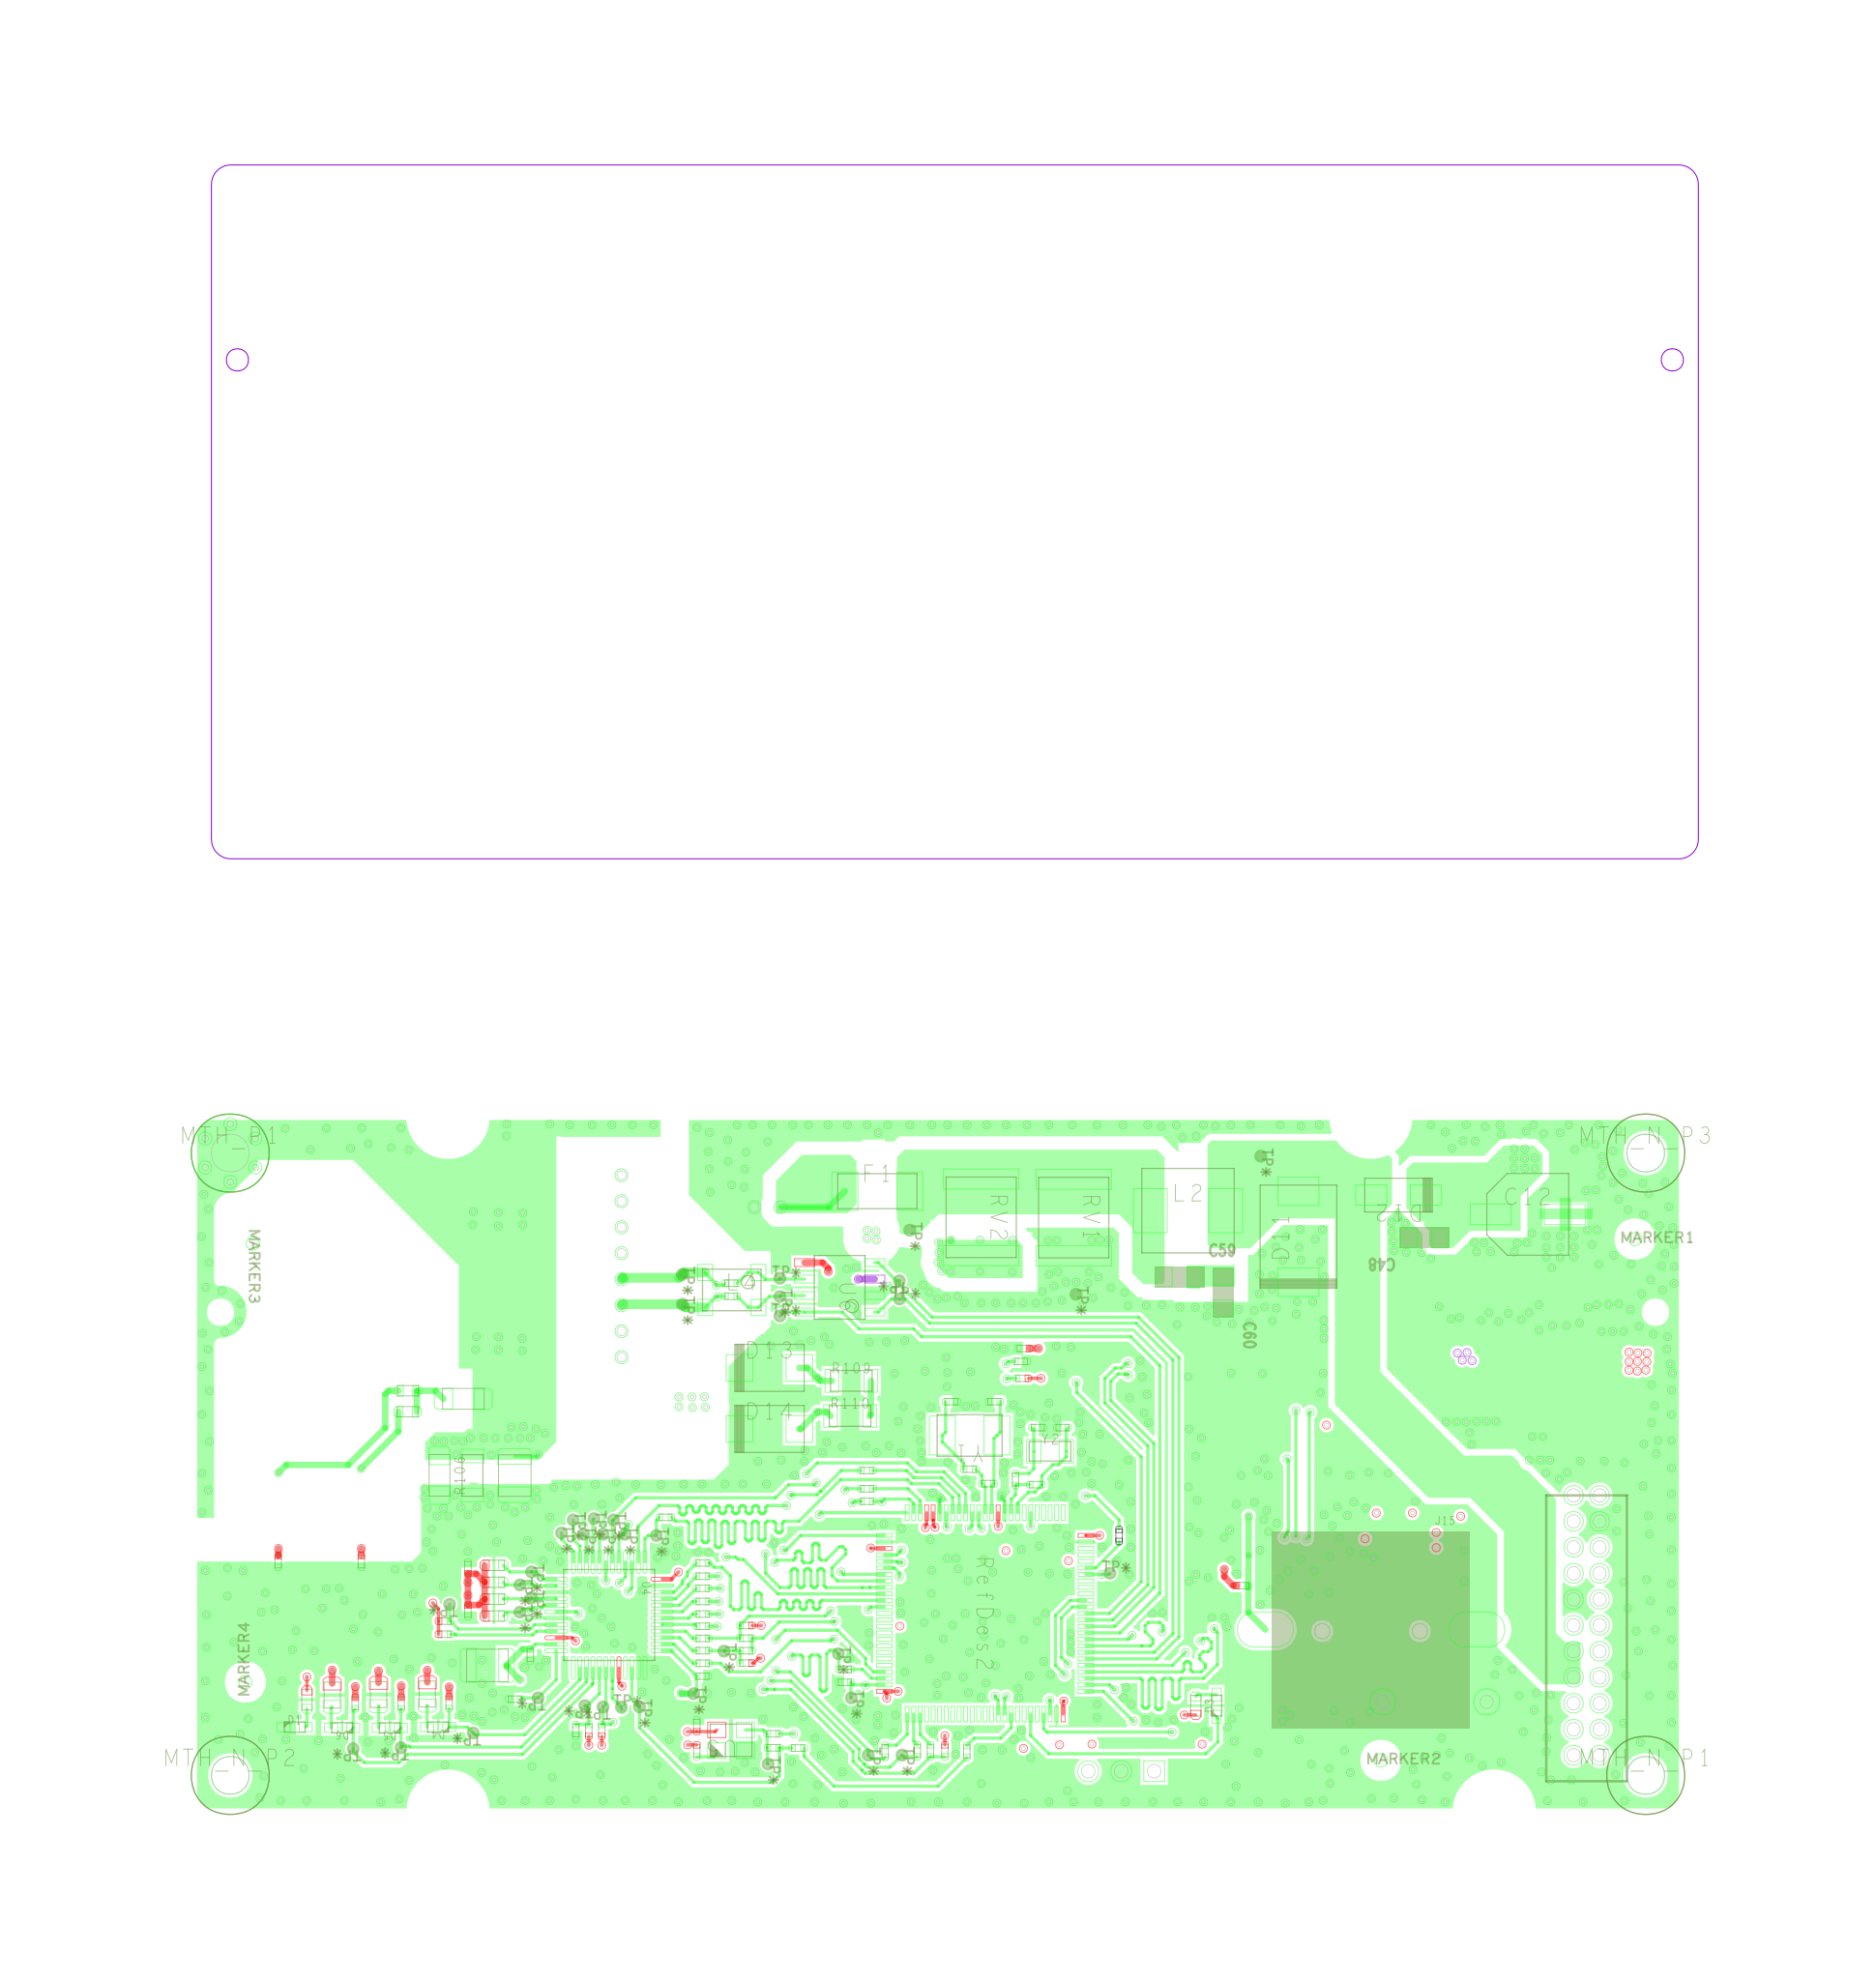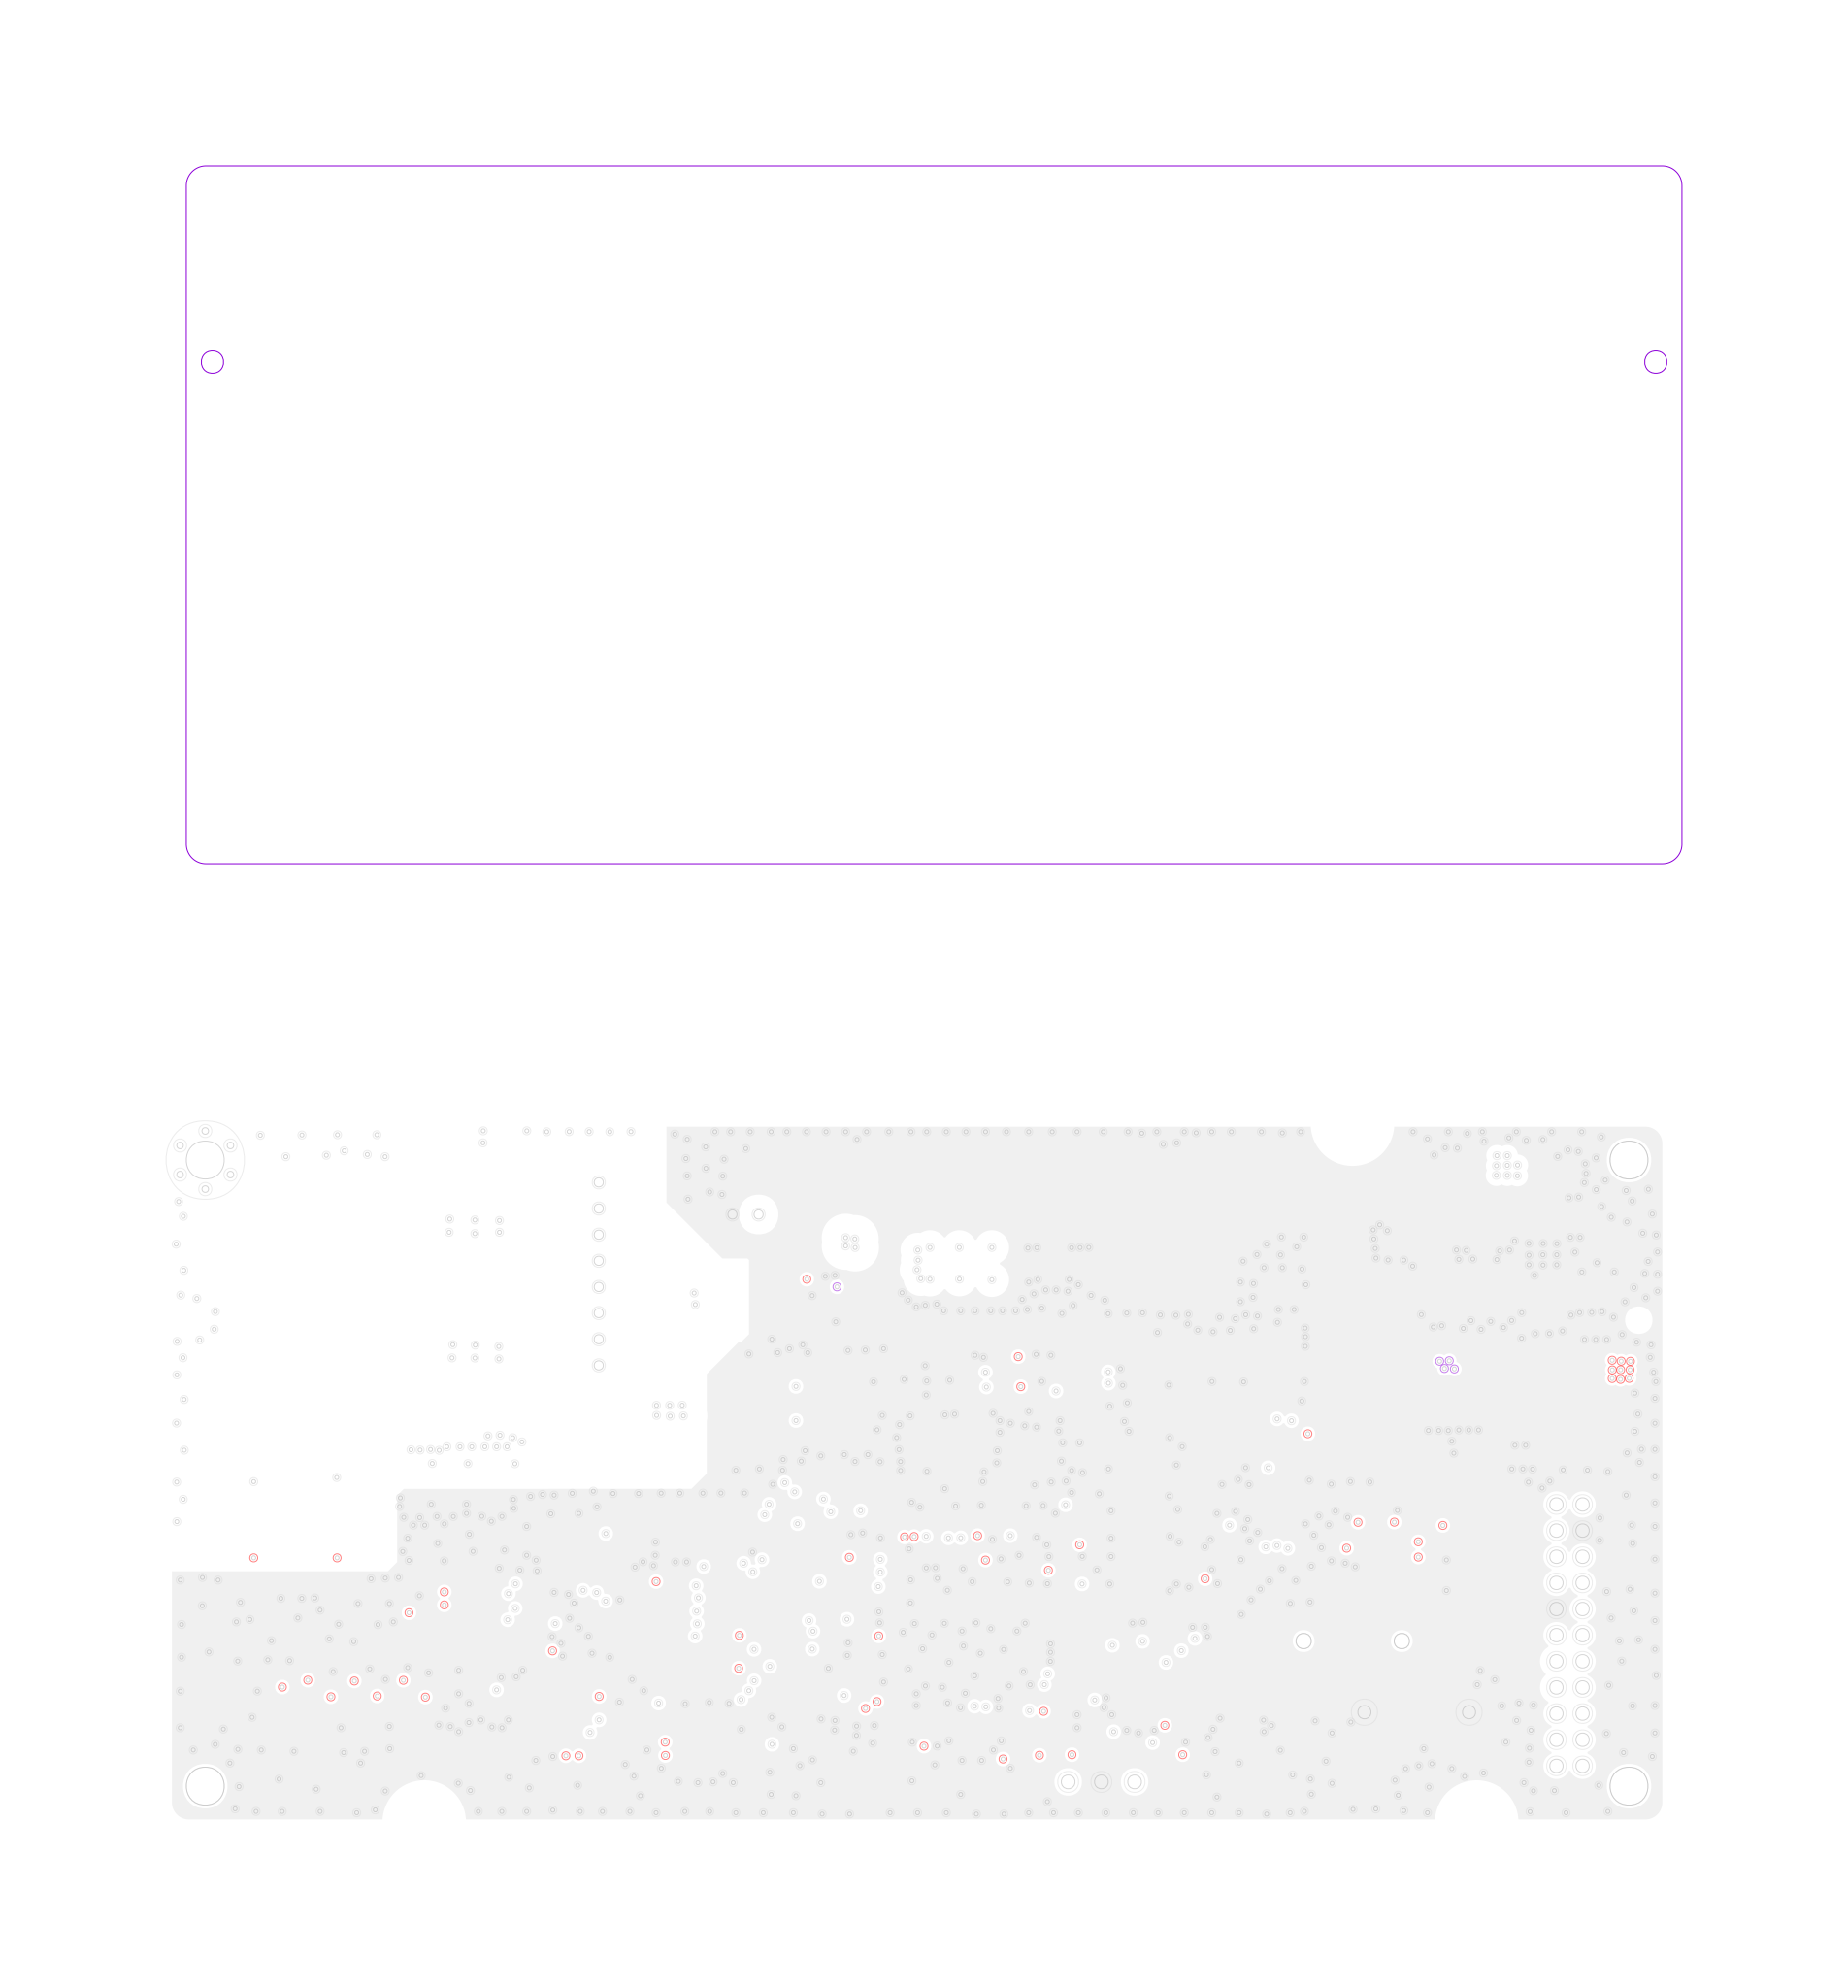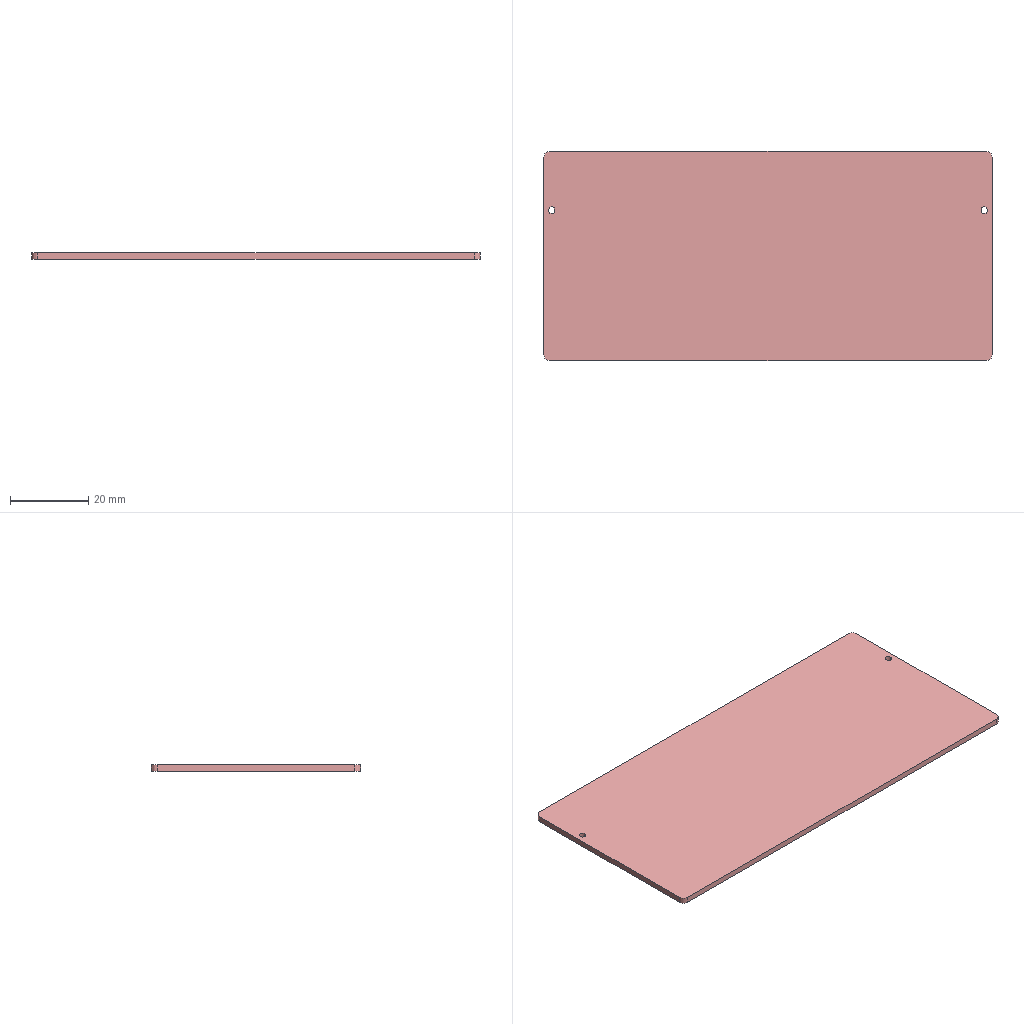Circuit board layout | Cadence Allegro | box 114.4 x 53.4 x 1.5 mm
Layer stack:
# Cadence Allegro layer stack of  (unit mm; from the constraint file cross-section; dielectric type: 0 not recorded (Allegro does not mark core vs prepreg), 3 surface material)
index,name,kind,layer,copper_thickness_mm,dielectric_type,dielectric_thickness_mm,dielectric_material,dielectric_constant
0,Top Surface,other,,,,,,
1,TOP,copper,TOP,0.03,,,,
2,Dielectric1,dielectric,,,0,0.5,FR-4,4.5
3,GND,copper,GND,0.03,,,,
4,Dielectric2,dielectric,,,0,0.5,FR-4,4.5
5,POWER,copper,POWER,0.03,,,,
6,Dielectric3,dielectric,,,0,0.48,FR-4,4.5
7,BOTTOM,copper,BOTTOM,0.03,,,,
8,Bottom Surface,other,,,,,,
# drill layer pairs: low layer,high layer
drill_pair,TOP,BOTTOM
Part placement:
REFDES,COMP_VALUE,SYM_NAME,SYM_X,SYM_Y,SYM_ROTATE,SYM_MIRROR
C1,8PF,C0402,154.5,96.5,180.000,NO
C2,8PF,C0402,157.8,96.5,0.000,NO
C3,6PF,C0402,161.145,94.5,0.000,NO
C4,6PF,C0402,163.045,94.5,180.000,NO
C6,22uf,C1210,192.63,95.39,90.000,YES
C7,22uf,C1210,187.28,101.31,0.000,YES
C8,.22uf,C0805,195.197,115.26,0.000,YES
C9,.1uf,C0402,193.15,101.71,270.000,YES
C10,4.7uf,C1210,202.062,114.475,180.000,YES
C11,.1uf,C0402,195.347,112.262,0.000,YES
C12,47uF,CAPAE630X770N,198.84,110.92,0.000,NO
C13,.1uf,C0402,160.058,100.595,180.000,NO
C14,10uf,C1210,118.8,76.2,180.000,NO
C15,.1uf,C0402,122.1,77,270.000,NO
C16,.1uf,C0402,145.6,107.2,180.000,YES
C17,.1uf,C0402,134.907,71.552,90.000,NO
C18,.1uf,C0402,125.6,71.2,270.000,NO
C19,10uf,C1210,196.08,95.43,90.000,YES
C20,1uf,C0603,194.39,101.9,270.000,YES
C21,.1uf,C0402,156.977,85.515,90.000,YES
C22,.1uf,C0402,191.8,87.47,270.000,YES
C23,2.2uf,C0603,185.52,87,0.000,YES
C24,.1uf,C0402,153.4,88,270.000,YES
C25,1uf,C0603,152.3,88.4,270.000,YES
C26,.1uf,C0402,164.7,86.2,0.000,YES
C27,.1uf,C0402,102.7,84.2,270.000,NO
C28,.1uf,C0402,158.088,88.097,270.000,YES
C29,.1uf,C0402,149.425,85.51,180.000,YES
C30,.1uf,C0402,153.936,85.518,90.000,YES
C31,.047uf,C0402,151.857,85.886,180.000,YES
C32,.047uf,C0402,151.857,81.745,180.000,YES
C33,.1uf,C0402,109.1,84.2,270.000,NO
C34,.047uf,C0402,151.84,83.793,180.000,YES
C35,.1uf,C0402,183.355,93.62,90.000,YES
C36,22uf,C1210,204.92,101.46,270.000,YES
C37,10uf,C1210,131.723,84.653,270.000,YES
C38,2.2uf,C0603,148.002,72.98,90.000,YES
C39,.1uf,C0402,134.301,84.145,270.000,YES
C40,.1uf,C0402,117.3,80.4,270.000,NO
C41,.1uf,C0402,149.518,72.64,90.000,YES
C42,.047uf,C0402,171.928,84.672,270.000,YES
C43,10uf,C1210,153.02,73.522,180.000,YES
C44,.1uf,C0402,162.54,72.507,0.000,YES
C45,.1uf,C0402,125.8,81.3,270.000,YES
C46,.1uf,C0402,117.3,83.7,90.000,NO
C47,2.2uf,C0603,161.285,74.382,0.000,YES
C48,.1uf,C0805,190.9,109.1,180.000,NO
C49,.1uf,C0402,124.484,77.668,0.000,YES
C50,.1uf,C0402,135.347,75.368,0.000,NO
C51,.1uf,C0402,129.637,73.805,180.000,YES
C52,1.5nF,C1206,116.948,96.718,0.000,NO
C53,47nf,C1210,120.903,90.81,90.000,NO
C54,.1uf,C0402,146.24,105.933,180.000,YES
C55,4700pf(NC),C0603,138.657,103.775,90.000,YES
C56,10nF,C1206,115.115,90.828,90.000,NO
C57,100PF,C0603,145.958,102.522,180.000,YES
C58,100PF,C0603,145.972,103.96,180.000,YES
C59,.1uf,C0805,172.048,106.11,0.000,NO
C60,.1uf,C0805,175.405,104.897,270.000,NO
D1,LED,LED0603,103.97,71.448,0.000,NO
D2,UFS08A2.8L04,SOIC127P600X175-8N,105.108,100.885,270.000,YES
D3,LED,LED0603,174.9,73.1,90.000,NO
D4,LED,LED0603,115.01,71.45,180.000,NO
D5,LED,LED0603,111.287,71.387,180.000,NO
D6,LED,LED0603,107.625,71.395,180.000,NO
D8,SMBJ10CA,SMB,147.205,97.103,270.000,YES
D9,SS26FL,SMA,199.49,100.78,180.000,YES
D10,SS26FL,SMA,196.67,107.65,270.000,YES
D11,TPSMC27CA,SMC,181.2,109.2,90.000,NO
D12,NRVA4007T3G,SMA,188.9,112.4,180.000,NO
D13,SMBJ10CA,SMB,140.5,99.1,0.000,NO
D14,SMBJ10CA,SMB,140.5,94.4,0.000,NO
F1,10A,FUSE10A,148.8,112.7,0.000,NO
GDT1,5kA,GDT5KA2P,152.705,108.942,0.000,YES
J15,BAT2,CR1220,186.785,78.834,0.000,NO
J17,532530870,532530870,129.116,106.926,180.000,YES
J18,532530270,532530270,140.342,111.471,270.000,YES
J19,2x11,CON2X11X200,202.366,69.286,90.000,NO
J20,3,CON3X254,170.1,68.06,0.000,YES
L1,6.8uH,SPM5030,191.18,106.38,0.000,YES
L2,22uH,SPM6530,172.7,111.2,0.000,NO
L3,51uH,CM320X450X150-4N,154.243,98.785,270.000,YES
L4,51uH,CM320X450X150-4N,137.6,105.1,270.000,NO
MARKER1,30mil,FIDMS0,207.09,109.02,0.000,NO
MARKER2,30mil,FIDMS0,187.54,68.89,0.000,NO
MARKER3,30mil,FIDMS0,100.75,108.67,270.000,NO
MARKER4,30mil,FIDMS0,100.18,74.918,90.000,NO
MARKER5,30mil,FIDMS0,185.08,112.74,0.000,YES
MARKER6,30mil,FIDMS0,178.09,71.59,270.000,YES
MARKER7,30mil,FIDMS0,100.75,108.65,0.000,YES
MARKER8,30mil,FIDMS0,100.18,74.918,0.000,YES
MTH_N_P1,D2.8no-plated,MTGNP600H280Z380P,207.916,67.736,0.000,NO
MTH_N_P2,D2.8no-plated,MTGNP600H280Z380P,99.016,67.736,0.000,NO
MTH_N_P3,D2.8no-plated,MTGNP600H280Z380P,207.916,115.636,0.000,NO
MTH_P1,D2.8plated,MTGP6000H280V6P,99.016,115.636,0.000,NO
R1,0R(NC),R0402,176.88,82.34,180.000,NO
R2,10k,R0402,190.7,87.47,90.000,YES
R3,10k,R0402,192.9,87.47,90.000,YES
R4,10k,R0402,194.7,87.47,90.000,YES
R5,10k,R0402,196.2,87.47,90.000,YES
R6,10k,R0402,189.3,87.47,90.000,YES
R7,10k,R0402,187.9,87.47,90.000,YES
R8,10k,R0402,200.542,103.71,90.000,YES
R9,68k,R0402,201.59,103.705,270.000,YES
R10,12k,R0402,202.635,103.72,90.000,YES
R11,16.9k,R0402,205.412,111.22,180.000,YES
R12,33R,R0402,148,91.2,180.000,NO
R13,0R,R0402,155.9,91.3,0.000,NO
R14,1k,R0603,104.912,73.565,270.000,NO
R15,1M,R0402,157.31,90.188,180.000,NO
R16,10M,R0402,160.99,90.112,0.000,NO
R17,0R,R0402,148,89.8,180.000,NO
R18,10k,R0402,197.7,87.47,90.000,YES
R19,0R,R0402,148.002,88.828,180.000,NO
R20,33R,R0402,132.5,87.6,180.000,NO
R21,33R,R0402,146.3,75.9,180.000,NO
R22,33R,R0402,135.351,84.081,180.000,NO
R23,0R(NC),R0402,146.3,74.9,180.000,NO
R24,33R,R0402,135.351,83.065,180.000,NO
R25,33R,R0402,135.351,82.138,180.000,NO
R26,2.2k,R0402,138.703,79.269,180.000,NO
R27,33R,R0402,135.351,81.122,180.000,NO
R28,0R,R0402,140.778,70.935,180.000,NO
R29,0R,R0402,138.703,78.294,180.000,NO
R30,33R,R0402,135.357,78.28,180.000,NO
R31,33R,R0402,149.4,69.6,270.000,NO
R32,33R,R0402,151.872,69.626,270.000,NO
R33,0R,R0402,152.888,69.626,90.000,NO
R34,10k,R0402,153.993,69.626,270.000,NO
R35,33R,R0402,155.683,69.575,90.000,NO
R36,0R,R0402,140.8,69.858,0.000,NO
R37,0R,R0402,138.703,77.329,180.000,NO
R38,33R,R0402,135.359,77.336,180.000,NO
R39,2.2k,R0402,138.703,76.376,180.000,NO
R40,33R,R0402,135.364,76.367,180.000,NO
R41,10k,R0402,159.958,98.295,180.000,NO
R42,10k,R0402,159.857,99.595,180.000,NO
R43,2.2k,R0402,115.5,78.6,180.000,NO
R44,2.2k,R0402,115.5,79.6,180.000,NO
R45,10k,R0402,134.907,69.62,90.000,NO
R46,0R,R0402,142.7,69.84,180.000,NO
R47,4.87k,R0402,120.9,73.6,180.000,NO
R48,10k,R0402,126.6,71.2,90.000,NO
R49,1.5k,R0402,127.6,71.2,90.000,NO
R50,4.7R,R1206,112.912,113.02,180.000,YES
R51,4.7R,R1206,112.907,109.525,180.000,YES
R52,4.7R,R1206,112.862,104.265,180.000,YES
R53,4.7R,R1206,112.88,100.933,180.000,YES
R57,10k,R0402,173.1,70.6,270.000,YES
R60,10k,R0402,168.78,70.6,90.000,YES
R62,10k,R0402,166,70.6,270.000,YES
R63,10k,R0402,163.5,70.6,270.000,YES
R65,10k,R0402,161,70.6,270.000,YES
R67,10k,R0402,158.018,85.49,270.000,YES
R68,0R,R0402,154.438,87.99,90.000,YES
R69,0R(NC),R0402,154.952,85.518,90.000,YES
R70,10k,R0402,164.708,84.25,180.000,YES
R71,1k,R0402,151.857,84.82,180.000,YES
R72,10k(NC),R0402,164.7,83.23,0.000,YES
R73,33R,R0402,167.4,86.2,90.000,NO
R74,1k,R0402,151.9,80.7,180.000,YES
R75,1k,R0402,190.67,112.32,90.000,YES
R76,10k,R0402,191.78,112.34,90.000,YES
R77,1k,R0402,185.591,96.978,180.000,YES
R78,10k,R0402,187.489,96.991,0.000,YES
R79,10k,R0402,181.197,93.612,270.000,YES
R80,1k,R0402,151.847,82.772,180.000,YES
R81,10k,R0402,182.23,93.605,90.000,YES
R82,10k(NC),R0402,149.385,79.225,0.000,YES
R83,10k,R0402,149.377,80.228,180.000,YES
R84,49.9R,R0603,119.3,83.9,180.000,NO
R85,49.9R,R0603,119.3,82.6,180.000,NO
R86,49.9R,R0603,119.3,81.3,180.000,NO
R87,1k,R0402,173.04,84.707,270.000,YES
R88,10k,R0402,175.037,84.692,270.000,YES
R89,49.9R,R0603,119.3,80,180.000,NO
R90,33R,R0402,135.36,80.153,180.000,NO
R91,75R,R0603,112.657,95.728,0.000,NO
R92,75R,R0603,112.695,97.34,0.000,NO
R93,1k,R0402,174.042,84.7,270.000,YES
R94,33R,R0402,135.363,79.213,180.000,NO
R95,1k,R0603,173.3,73.1,90.000,NO
R96,2.2k,R0402,115.855,73.335,90.000,NO
R97,390R,R0805,114.17,74,90.000,NO
R98,2.2k,R0402,112.17,73.295,90.000,NO
R99,390R,R0805,110.422,73.957,90.000,NO
R101,62R(NC),R1206,142.12,105.112,0.000,YES
R102,62R(NC),R1206,142.12,102.705,0.000,YES
R103,2.2k,R0402,108.63,73.293,90.000,NO
R104,390R,R0805,106.86,73.907,90.000,NO
R106,1M,R1206,117.655,90.82,90.000,NO
R109,62R,R1206,146.8,98.1,0.000,NO
R110,62R,R1206,146.7,95.4,0.000,NO
R111,4.7R,R1206,141.852,98.315,0.000,YES
R112,4.7R,R1206,141.882,95.705,0.000,YES
R113,10R,R0402,159.43,90.507,90.000,NO
R114,0R(NC),R0402,137.555,105.618,180.000,NO
R115,0R(NC),R0402,137.545,104.61,180.000,NO
RT1,10K,R0603,179.425,93.045,0.000,YES
RV1,47V,R2220,163.905,110.668,270.000,NO
RV2,47V,R2220,156.79,110.69,270.000,NO
RV3,47V,R2220,160.925,108.942,180.000,YES
T1,HR641680E,H1102,105.897,88.26,270.000,YES
TF1,TF-01A,TF-01A,198.49,73.39,0.000,YES
TP1,TP,TPAD_30MIL,164.084,104.763,270.000,NO
TP2,TP,TPAD_30MIL,184.827,94.356,180.000,YES
TP3,TP,TPAD_30MIL,205.374,105.758,180.000,YES
TP4,TP,TPAD_30MIL,205.256,109.746,90.000,YES
TP5,TP,TPAD_30MIL,194.801,85.766,90.000,YES
TP6,TP,TPAD_30MIL,190.699,85.774,270.000,YES
TP7,TP,TPAD_30MIL,187.899,85.874,270.000,YES
TP8,TP,TPAD_30MIL,192.904,85.871,180.000,YES
TP9,TP,TPAD_30MIL,189.299,85.874,270.000,YES
TP10,TP,TPAD_30MIL,196.199,85.774,270.000,YES
TP11,TP,TPAD_30MIL,129.399,86.296,270.000,NO
TP12,TP,TPAD_30MIL,198.161,113.814,180.000,YES
TP13,TP,TPAD_30MIL,156.804,87.669,90.000,YES
TP14,TP,TPAD_30MIL,193.149,98.794,270.000,YES
TP15,TP,TPAD_30MIL,197.699,85.774,270.000,YES
TP16,TP,TPAD_30MIL,102.838,96.323,90.000,YES
TP17,TP,TPAD_30MIL,197.288,112.183,90.000,YES
TP18,TP,TPAD_30MIL,104.328,96.31,90.000,YES
TP19,TP,TPAD_30MIL,193.681,112.196,90.000,YES
TP20,TP,TPAD_30MIL,166.704,83.299,0.000,NO
TP21,TP,TPAD_30MIL,105.828,96.26,90.000,YES
TP22,TP,TPAD_30MIL,167.161,99.296,180.000,YES
TP23,TP,TPAD_30MIL,167.462,100.696,180.000,YES
TP24,TP,TPAD_30MIL,107.255,96.272,90.000,YES
TP25,TP,TPAD_30MIL,126.999,87.496,270.000,NO
TP26,TP,TPAD_30MIL,127.699,86.296,270.000,NO
TP27,TP,TPAD_30MIL,167.357,97.699,270.000,YES
TP28,TP,TPAD_30MIL,126.199,86.296,270.000,NO
TP29,TP,TPAD_30MIL,145.799,77.096,270.000,NO
TP30,TP,TPAD_30MIL,125.399,87.396,270.000,NO
TP31,TP,TPAD_30MIL,128.499,87.396,270.000,NO
TP32,TP,TPAD_30MIL,124.499,86.396,270.000,NO
TP33,TP,TPAD_30MIL,133.799,106.296,270.000,NO
TP34,TP,TPAD_30MIL,131.799,86.196,270.000,NO
TP35,TP,TPAD_30MIL,122.199,83.396,270.000,NO
TP36,TP,TPAD_30MIL,121.299,82.396,270.000,NO
TP37,TP,TPAD_30MIL,122.199,81.396,270.000,NO
TP38,TP,TPAD_30MIL,178.299,115.396,270.000,NO
TP39,TP,TPAD_30MIL,121.299,80.296,270.000,NO
TP40,TP,TPAD_30MIL,133.799,103.996,270.000,NO
TP41,TP,TPAD_30MIL,146.799,73.696,270.000,NO
TP42,TP,TPAD_30MIL,186.001,95.744,270.000,YES
TP43,TP,TPAD_30MIL,182.201,91.919,0.000,YES
TP44,TP,TPAD_30MIL,163.416,74.351,90.000,YES
TP45,TP,TPAD_30MIL,189.276,111.949,0.000,YES
TP46,TP,TPAD_30MIL,176.369,85.199,0.000,YES
TP47,TP,TPAD_30MIL,157.999,98.004,270.000,YES
TP48,TP,TPAD_30MIL,136.999,77.296,270.000,NO
TP49,TP,TPAD_30MIL,130.499,72.996,270.000,NO
TP50,TP,TPAD_30MIL,150.699,69.296,270.000,NO
TP51,TP,TPAD_30MIL,148.099,69.296,270.000,NO
TP52,TP,TPAD_30MIL,150.496,105.801,180.000,NO
TP53,TP,TPAD_30MIL,140.394,68.603,270.000,NO
TP55,TP,TPAD_30MIL,134.672,74.023,270.000,NO
TP56,TP,TPAD_30MIL,157.999,99.404,270.000,YES
TP57,TP,TPAD_30MIL,115.896,80.901,180.000,NO
TP58,TP,TPAD_30MIL,141.304,105.999,0.000,NO
TP59,TP,TPAD_30MIL,122.696,73.701,180.000,NO
TP60,TP,TPAD_30MIL,117.706,71.001,180.000,NO
TP61,TP,TPAD_30MIL,141.299,104.596,270.000,NO
TP62,TP,TPAD_30MIL,103.114,105.736,90.000,YES
TP63,TP,TPAD_30MIL,104.465,105.728,90.000,YES
TP64,TP,TPAD_30MIL,105.814,105.711,90.000,YES
TP65,TP,TPAD_30MIL,107.189,105.674,90.000,YES
TP66,TP,TPAD_30MIL,129.104,72.999,0.000,NO
TP67,TP,TPAD_30MIL,126.296,73.101,180.000,NO
TP68,TP,TPAD_30MIL,112.151,69.864,180.000,NO
TP69,TP,TPAD_30MIL,150.504,104.399,0.000,NO
TP70,TP,TPAD_30MIL,150.501,97.396,90.000,YES
TP71,TP,TPAD_30MIL,150.401,99.696,90.000,YES
TP72,TP,TPAD_30MIL,127.696,73.001,180.000,NO
TP73,TP,TPAD_30MIL,141.304,103.099,0.000,NO
TP74,TP,TPAD_30MIL,108.474,69.789,180.000,NO
TP76,TP,TPAD_30MIL,151.299,109.696,270.000,NO
U1,LMR16010PDDAR,DDA0008E_N,201.31,108.49,90.000,YES
U2,STM32F407VET6,LQFP100-14X14MM,157.094,80.203,270.000,NO
U3,MAX3485EESA,SOIC127P600X175-8N,162.657,98.895,0.000,YES
U4,DP83848IVVX/NOPB,VBH48A_N,128.167,80.081,270.000,NO
U5,ECS-3225MV-500-CN-TR,OSCSC210P250X320X110-4N,137.547,70.436,90.000,NO
U6,TJA1044GT/3Z,SOIC127P600X175-8N,145.9,105.3,180.000,NO
U8,5kA,GDT3P,119.662,110.582,90.000,YES
U9,5kA,GDT3P,119.693,101,90.000,YES
U10,5kA,GDT3P,135.708,96.375,270.000,YES
U11,AMS1117-3.3,SOT223,202.59,95.21,180.000,YES
Y1,NX5032GA-25.000M,XTAL500X320X150N,155.9,93.9,180.000,NO
Y2,XDMCZLNDDF-32.768K,XTAL320X150X90N,162.085,92.679,0.000,NO
Pad and via stacks:
# Allegro (Cadence) via spans and padstacks; design units: ("millimeters" 4 10000)
# via spans: padstack,start_layer,end_layer,net_example,count
# Allegro padstack definitions: name,start_layer,end_layer,drill,plating,holeType,type
TPAD_30MIL,"ETCH/TOP","ETCH/TOP",0.0,"PLATED","none","smd"
PCM40S120,"ETCH/TOP","ETCH/TOP",0.0,"PLATED","none","smd"
S205,"ETCH/TOP","ETCH/TOP",0.0,"PLATED","none","smd"
R580_125,"ETCH/TOP","ETCH/TOP",0.0,"PLATED","none","smd"
R240_155,"ETCH/TOP","ETCH/TOP",0.0,"PLATED","none","smd"
R580_155,"ETCH/TOP","ETCH/TOP",0.0,"PLATED","none","smd"
R315_220,"ETCH/TOP","ETCH/TOP",0.0,"PLATED","none","smd"
R340_260,"ETCH/TOP","ETCH/TOP",0.0,"PLATED","none","smd"
R295_200,"ETCH/TOP","ETCH/TOP",0.0,"PLATED","none","smd"
R315_160,"ETCH/TOP","ETCH/TOP",0.0,"PLATED","none","smd"
R125_115,"ETCH/TOP","ETCH/TOP",0.0,"PLATED","none","smd"
R10240570000200A,"ETCH/TOP","ETCH/TOP",0.0,"PLATED","none","smd"
R10941220000200A,"ETCH/TOP","ETCH/TOP",0.0,"PLATED","none","smd"
R215_210,"ETCH/TOP","ETCH/TOP",0.0,"PLATED","none","smd"
R155_60,"ETCH/TOP","ETCH/TOP",0.0,"PLATED","none","smd"
R100_70,"ETCH/TOP","ETCH/TOP",0.0,"PLATED","none","smd"
R515_110,"ETCH/TOP","ETCH/TOP",0.0,"PLATED","none","smd"
SMD56X20,"ETCH/TOP","ETCH/TOP",0.0,"PLATED","none","smd"
R215_95,"ETCH/TOP","ETCH/TOP",0.0,"PLATED","none","smd"
R325_215,"ETCH/TOP","ETCH/TOP",0.0,"PLATED","none","smd"
RX47Y12D0T,"ETCH/TOP","ETCH/TOP",0.0,"PLATED","none","smd"
R215_130,"ETCH/TOP","ETCH/TOP",0.0,"PLATED","none","smd"
R300_200,"ETCH/TOP","ETCH/TOP",0.0,"PLATED","none","smd"
O1011810689000000P,"ETCH/TOP","ETCH/TOP",0.0,"PLATED","none","smd"
R120_110,"ETCH/TOP","ETCH/TOP",0.0,"PLATED","none","smd"
R614_253,"ETCH/TOP","ETCH/TOP",0.0,"PLATED","none","smd"
SMD12X20,"ETCH/TOP","ETCH/TOP",0.0,"PLATED","none","smd"
SMD12X14,"ETCH/TOP","ETCH/TOP",0.0,"PLATED","none","smd"
SMD07X13,"ETCH/TOP","ETCH/TOP",0.0,"PLATED","none","smd"
B195_75,"ETCH/TOP","ETCH/TOP",0.0,"PLATED","none","smd"
R175_105,"ETCH/TOP","ETCH/TOP",0.0,"PLATED","none","smd"
R100_95,"ETCH/TOP","ETCH/TOP",0.0,"PLATED","none","smd"
SR60X100,"ETCH/TOP","ETCH/TOP",0.0,"PLATED","none","smd"
SR60X50,"ETCH/TOP","ETCH/TOP",0.0,"PLATED","none","smd"
SR36X32,"ETCH/TOP","ETCH/TOP",0.0,"PLATED","none","smd"
SR600X500M,"ETCH/TOP","ETCH/TOP",0.0,"PLATED","none","smd"
R0402,"ETCH/TOP","ETCH/TOP",0.0,"NON_PLATED","none","smd"
C1206,"ETCH/TOP","ETCH/TOP",0.0,"NON_PLATED","none","smd"
S160H105T155_190_40,"ETCH/TOP","ETCH/BOTTOM",1.049,"PLATED","circle_drill","through"
C160H105T155_190_40,"ETCH/TOP","ETCH/BOTTOM",1.049,"PLATED","circle_drill","through"
C550HN240,"ETCH/TOP","ETCH/BOTTOM",2.4,"NON_PLATED","circle_drill","through"
THRUD1,"ETCH/TOP","ETCH/BOTTOM",1.001,"PLATED","circle_drill","through"
C550H240,"ETCH/TOP","ETCH/BOTTOM",2.4,"PLATED","circle_drill","through"
V100H50,"ETCH/TOP","ETCH/BOTTOM",0.5004,"PLATED","circle_drill","through"
VIA024D012,"ETCH/TOP","ETCH/BOTTOM",0.3048,"PLATED","circle_drill","through"
VIA032D014,"ETCH/TOP","ETCH/BOTTOM",0.3556,"PLATED","circle_drill","through"
C0402,"ETCH/TOP","ETCH/TOP",0.0,"NON_PLATED","none","smd"
C1210,"ETCH/TOP","ETCH/TOP",0.0,"NON_PLATED","none","smd"
C0603,"ETCH/TOP","ETCH/TOP",0.0,"NON_PLATED","none","smd"
R0805,"ETCH/TOP","ETCH/TOP",0.0,"NON_PLATED","none","smd"
R1P2X1P4,"ETCH/TOP","ETCH/TOP",0.0,"PLATED","none","smd"
R1P1X1P8,"ETCH/TOP","ETCH/TOP",0.0,"PLATED","none","smd"
C600H280,"ETCH/TOP","ETCH/BOTTOM",2.9,"PLATED","circle_drill","through"
C600H280Z380P,"ETCH/TOP","ETCH/BOTTOM",2.8,"PLATED","circle_drill","through"
PTH_C1P02C1P5,"ETCH/TOP","ETCH/BOTTOM",1.02,"PLATED","circle_drill","through"
PTH_C1P02_SQ1P5,"ETCH/TOP","ETCH/BOTTOM",1.02,"PLATED","circle_drill","through"
C600NPH280,"ETCH/TOP","ETCH/BOTTOM",2.9,"NON_PLATED","circle_drill","through"
SMD4R3X2R7MMOB,"ETCH/TOP","ETCH/TOP",0.0,"NON_PLATED","none","smd"
NPAD46,"ETCH/TOP","ETCH/BOTTOM",1.168,"NON_PLATED","circle_drill","through"
PTH_C0P7C1P0,"ETCH/TOP","ETCH/BOTTOM",0.7,"PLATED","circle_drill","through"
C150,"ETCH/TOP","ETCH/BOTTOM",1.0,"PLATED","circle_drill","through"
Design rules, without the lines most boards share, first 11 of 42 lines:
# Cadence Allegro design rules of  (from the Constraint Manager export constraints.dcfx, design unit mm; typed fields in mm)
# columns: name | kind | enabled | priority | scope1 | scope2 | descriptor | typed fields (field=value)
# Allegro precedence (priority 1 wins): 1 Region class-to-class, 2 Region class, 3 Region, 4 class-to-class, 5 DiffPair/Bus/NetGroup override, 6 NetClass, 7 constraint set (CSet) default
# per-layer values are written LAYER=value in the descriptor and LAYER:mm in the typed field; a maximum of 0 means no limit set
# --- net classes (and buses / net groups) ---
HV | NetClass | enabled | 6 | N00275, POWER_IN, N02752, VOUT | All | Net Class (members: 4 Net) |
HV_PH | NetClass | enabled | 6 | N00275, POWER_IN, N02752, VOUT | All | Net Class (members: 4 Net) |
HV | NetGroup | enabled | 5 | N00275, N02752, POWER_IN | All | NetGroup (SpacingCSet=EARTH) (members: 3 Net) | spacingcset=EARTH
# --- track widths, neck and differential-pair gap (physical constraint sets) ---
1MM | PhysicalCSet | enabled | 7 | not referenced | All | Physical Constraint (Min Line Width=0.254mm) (Max Line Width=0mm) (Min Neck Width=0.254mm) (Max Neck Length=0mm) (DiffPair Primary Gap=0mm) (DiffPair Neck Gap=0mm) (DiffPair Min Space=0.2032mm) (DiffPair Coupled +Tol=0mm) (DiffPair Coupled -Tol=0mm) (Min BB Via Stagger=0.254mm) (Max BB Via Stagger=0mm) (T-junctions=ANYWHERE) (Pad-pad direct connect=ALL_ALLOWED) (Allowed vias=VIA024D012, VIA032D014) | min_line_width=0.254 min_neck_width=0.254 min_bvia_stagger=0.254 max_bvia_stagger=0 ts_allowed=ANYWHERE diffp_primary_gap=0 diffp_neck_gap=0 max_line_width=0 maximum_neck_length=0 pad_pad_direct_connect=ALL_ALLOWED allow_on_etch_subclass=TRUE diffp_coupled_plus=0 diffp_coupled_minus=0 diffp_min_space=0.2032 vias=VIA024D012,VIA032D014
DIFF | PhysicalCSet | enabled | 7 | DiffPair(1): DP6 | All | Physical Constraint (Min Line Width=0.254mm) (Max Line Width=0mm) (Min Neck Width=0.254mm) (Max Neck Length=0mm) (DiffPair Primary Gap=0.254mm) (DiffPair Neck Gap=0mm) (DiffPair Min Space=0.2032mm) (DiffPair Coupled +Tol=0mm) (DiffPair Coupled -Tol=0mm) (Min BB Via Stagger=0.254mm) (Max BB Via Stagger=0mm) (T-junctions=ANYWHERE) (Pad-pad direct connect=ALL_ALLOWED) (Allowed vias=VIA024D012, VIA032D014) | min_line_width=0.254 min_neck_width=0.254 min_bvia_stagger=0.254 max_bvia_stagger=0 ts_allowed=ANYWHERE diffp_primary_gap=0.254 diffp_neck_gap=0 max_line_width=0 maximum_neck_length=0 pad_pad_direct_connect=ALL_ALLOWED allow_on_etch_subclass=TRUE diffp_coupled_plus=0 diffp_coupled_minus=0 diffp_min_space=0.2032 vias=VIA024D012,VIA032D014